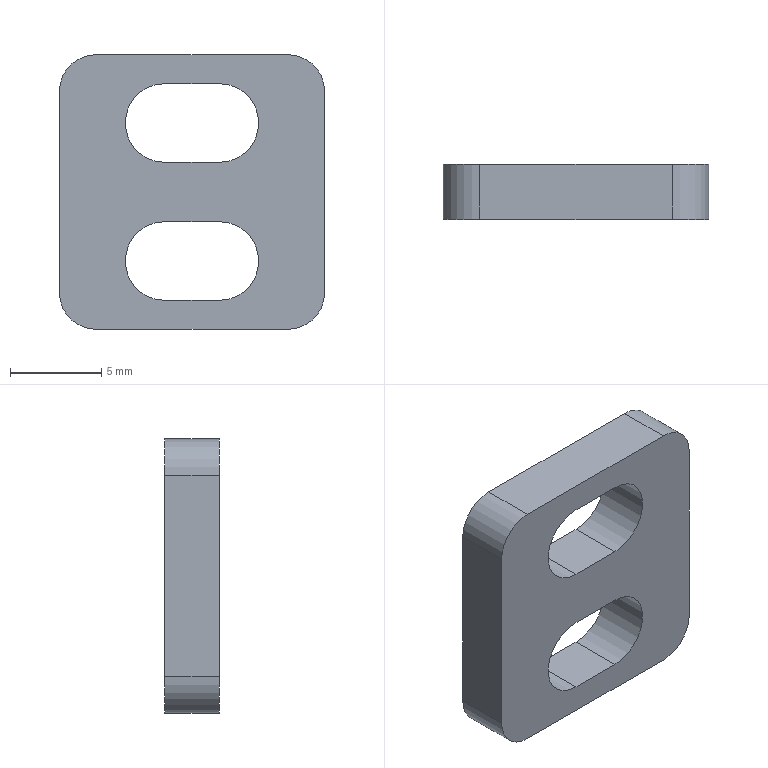Part | SolidWorks | features Extrusion 1, Fillet 1, ICE 1 | 1 solid | 18 faces | box 14.5 x 3 x 15 mm | volume 477.667 mm3 | plane 10 | cylinder 8 | commonest cylinder face diameters 4 x4 4.3 x4
STEP:
#1=CARTESIAN_POINT('',(7.25,0.,5.5));
#2=VERTEX_POINT('',#1);
#3=CARTESIAN_POINT('',(7.25,0.,-5.5));
#4=VERTEX_POINT('',#3);
#5=CARTESIAN_POINT('',(7.25,0.,-7.5));
#6=DIRECTION('',(0.,0.,-1.));
#7=VECTOR('',#6,1000.);
#8=LINE('',#5,#7);
#9=EDGE_CURVE('',#2,#4,#8,.T.);
#10=ORIENTED_EDGE('',*,*,#9,.T.);
#11=CARTESIAN_POINT('',(7.25,3.,-5.5));
#12=VERTEX_POINT('',#11);
#13=CARTESIAN_POINT('',(7.25,3.,-5.5));
#14=DIRECTION('',(0.,1.,0.));
#15=VECTOR('',#14,1000.);
#16=LINE('',#13,#15);
#17=EDGE_CURVE('',#4,#12,#16,.T.);
#18=ORIENTED_EDGE('',*,*,#17,.T.);
#19=CARTESIAN_POINT('',(7.25,3.,5.5));
#20=VERTEX_POINT('',#19);
#21=CARTESIAN_POINT('',(7.25,3.,-7.5));
#22=DIRECTION('',(0.,0.,-1.));
#23=VECTOR('',#22,1000.);
#24=LINE('',#21,#23);
#25=EDGE_CURVE('',#20,#12,#24,.T.);
#26=ORIENTED_EDGE('',*,*,#25,.F.);
#27=CARTESIAN_POINT('',(7.25,3.,5.5));
#28=DIRECTION('',(0.,-1.,0.));
#29=VECTOR('',#28,1000.);
#30=LINE('',#27,#29);
#31=EDGE_CURVE('',#20,#2,#30,.T.);
#32=ORIENTED_EDGE('',*,*,#31,.T.);
#33=EDGE_LOOP('',(#10,#18,#26,#32));
#34=FACE_OUTER_BOUND('',#33,.T.);
#35=CARTESIAN_POINT('',(7.25,3.,-7.5));
#36=DIRECTION('',(-1.,0.,0.));
#37=DIRECTION('',(0.,0.,1.));
#38=AXIS2_PLACEMENT_3D('',#35,#36,#37);
#39=PLANE('',#38);
#40=ADVANCED_FACE('',(#34),#39,.F.);
#41=CARTESIAN_POINT('',(5.25,3.,-7.5));
#42=VERTEX_POINT('',#41);
#43=CARTESIAN_POINT('',(-5.25,3.,-7.5));
#44=VERTEX_POINT('',#43);
#45=CARTESIAN_POINT('',(-7.25,3.,-7.5));
#46=DIRECTION('',(-1.,0.,0.));
#47=VECTOR('',#46,1000.);
#48=LINE('',#45,#47);
#49=EDGE_CURVE('',#42,#44,#48,.T.);
#50=ORIENTED_EDGE('',*,*,#49,.F.);
#51=CARTESIAN_POINT('',(5.25,0.,-7.5));
#52=VERTEX_POINT('',#51);
#53=CARTESIAN_POINT('',(5.25,3.,-7.5));
#54=DIRECTION('',(0.,-1.,0.));
#55=VECTOR('',#54,1000.);
#56=LINE('',#53,#55);
#57=EDGE_CURVE('',#42,#52,#56,.T.);
#58=ORIENTED_EDGE('',*,*,#57,.T.);
#59=CARTESIAN_POINT('',(-5.25,0.,-7.5));
#60=VERTEX_POINT('',#59);
#61=CARTESIAN_POINT('',(-7.25,0.,-7.5));
#62=DIRECTION('',(-1.,0.,0.));
#63=VECTOR('',#62,1000.);
#64=LINE('',#61,#63);
#65=EDGE_CURVE('',#52,#60,#64,.T.);
#66=ORIENTED_EDGE('',*,*,#65,.T.);
#67=CARTESIAN_POINT('',(-5.25,3.,-7.5));
#68=DIRECTION('',(0.,1.,0.));
#69=VECTOR('',#68,1000.);
#70=LINE('',#67,#69);
#71=EDGE_CURVE('',#60,#44,#70,.T.);
#72=ORIENTED_EDGE('',*,*,#71,.T.);
#73=EDGE_LOOP('',(#50,#58,#66,#72));
#74=FACE_OUTER_BOUND('',#73,.T.);
#75=CARTESIAN_POINT('',(-7.25,3.,-7.5));
#76=DIRECTION('',(0.,0.,1.));
#77=DIRECTION('',(1.,0.,0.));
#78=AXIS2_PLACEMENT_3D('',#75,#76,#77);
#79=PLANE('',#78);
#80=ADVANCED_FACE('',(#74),#79,.F.);
#81=CARTESIAN_POINT('',(-7.25,3.,-5.5));
#82=VERTEX_POINT('',#81);
#83=CARTESIAN_POINT('',(-7.25,3.,5.5));
#84=VERTEX_POINT('',#83);
#85=CARTESIAN_POINT('',(-7.25,3.,-7.5));
#86=DIRECTION('',(0.,0.,1.));
#87=VECTOR('',#86,1000.);
#88=LINE('',#85,#87);
#89=EDGE_CURVE('',#82,#84,#88,.T.);
#90=ORIENTED_EDGE('',*,*,#89,.F.);
#91=CARTESIAN_POINT('',(-7.25,0.,-5.5));
#92=VERTEX_POINT('',#91);
#93=CARTESIAN_POINT('',(-7.25,3.,-5.5));
#94=DIRECTION('',(0.,-1.,0.));
#95=VECTOR('',#94,1000.);
#96=LINE('',#93,#95);
#97=EDGE_CURVE('',#82,#92,#96,.T.);
#98=ORIENTED_EDGE('',*,*,#97,.T.);
#99=CARTESIAN_POINT('',(-7.25,0.,5.5));
#100=VERTEX_POINT('',#99);
#101=CARTESIAN_POINT('',(-7.25,0.,-7.5));
#102=DIRECTION('',(0.,0.,1.));
#103=VECTOR('',#102,1000.);
#104=LINE('',#101,#103);
#105=EDGE_CURVE('',#92,#100,#104,.T.);
#106=ORIENTED_EDGE('',*,*,#105,.T.);
#107=CARTESIAN_POINT('',(-7.25,3.,5.5));
#108=DIRECTION('',(0.,1.,0.));
#109=VECTOR('',#108,1000.);
#110=LINE('',#107,#109);
#111=EDGE_CURVE('',#100,#84,#110,.T.);
#112=ORIENTED_EDGE('',*,*,#111,.T.);
#113=EDGE_LOOP('',(#90,#98,#106,#112));
#114=FACE_OUTER_BOUND('',#113,.T.);
#115=CARTESIAN_POINT('',(-7.25,3.,-7.5));
#116=DIRECTION('',(1.,0.,0.));
#117=DIRECTION('',(0.,0.,-1.));
#118=AXIS2_PLACEMENT_3D('',#115,#116,#117);
#119=PLANE('',#118);
#120=ADVANCED_FACE('',(#114),#119,.F.);
#121=CARTESIAN_POINT('',(-5.25,3.,7.5));
#122=VERTEX_POINT('',#121);
#123=CARTESIAN_POINT('',(5.25,3.,7.5));
#124=VERTEX_POINT('',#123);
#125=CARTESIAN_POINT('',(-7.25,3.,7.5));
#126=DIRECTION('',(1.,0.,0.));
#127=VECTOR('',#126,1000.);
#128=LINE('',#125,#127);
#129=EDGE_CURVE('',#122,#124,#128,.T.);
#130=ORIENTED_EDGE('',*,*,#129,.F.);
#131=CARTESIAN_POINT('',(-5.25,0.,7.5));
#132=VERTEX_POINT('',#131);
#133=CARTESIAN_POINT('',(-5.25,3.,7.5));
#134=DIRECTION('',(0.,-1.,0.));
#135=VECTOR('',#134,1000.);
#136=LINE('',#133,#135);
#137=EDGE_CURVE('',#122,#132,#136,.T.);
#138=ORIENTED_EDGE('',*,*,#137,.T.);
#139=CARTESIAN_POINT('',(5.25,0.,7.5));
#140=VERTEX_POINT('',#139);
#141=CARTESIAN_POINT('',(-7.25,0.,7.5));
#142=DIRECTION('',(1.,0.,0.));
#143=VECTOR('',#142,1000.);
#144=LINE('',#141,#143);
#145=EDGE_CURVE('',#132,#140,#144,.T.);
#146=ORIENTED_EDGE('',*,*,#145,.T.);
#147=CARTESIAN_POINT('',(5.25,3.,7.5));
#148=DIRECTION('',(0.,1.,0.));
#149=VECTOR('',#148,1000.);
#150=LINE('',#147,#149);
#151=EDGE_CURVE('',#140,#124,#150,.T.);
#152=ORIENTED_EDGE('',*,*,#151,.T.);
#153=EDGE_LOOP('',(#130,#138,#146,#152));
#154=FACE_OUTER_BOUND('',#153,.T.);
#155=CARTESIAN_POINT('',(-7.25,3.,7.5));
#156=DIRECTION('',(0.,0.,-1.));
#157=DIRECTION('',(-1.,0.,0.));
#158=AXIS2_PLACEMENT_3D('',#155,#156,#157);
#159=PLANE('',#158);
#160=ADVANCED_FACE('',(#154),#159,.F.);
#161=CARTESIAN_POINT('',(1.5,3.,5.922));
#162=VERTEX_POINT('',#161);
#163=CARTESIAN_POINT('',(1.5,3.,1.622));
#164=VERTEX_POINT('',#163);
#165=CARTESIAN_POINT('',(1.5,3.,3.772));
#166=DIRECTION('',(0.,1.,0.));
#167=DIRECTION('',(0.,0.,1.));
#168=AXIS2_PLACEMENT_3D('',#165,#166,#167);
#169=CIRCLE('',#168,2.15);
#170=EDGE_CURVE('',#162,#164,#169,.T.);
#171=ORIENTED_EDGE('',*,*,#170,.F.);
#172=CARTESIAN_POINT('',(-1.5,3.,5.922));
#173=VERTEX_POINT('',#172);
#174=CARTESIAN_POINT('',(0.,3.,5.922));
#175=DIRECTION('',(1.,0.,0.));
#176=VECTOR('',#175,1000.);
#177=LINE('',#174,#176);
#178=EDGE_CURVE('',#173,#162,#177,.T.);
#179=ORIENTED_EDGE('',*,*,#178,.F.);
#180=CARTESIAN_POINT('',(-1.5,3.,1.622));
#181=VERTEX_POINT('',#180);
#182=CARTESIAN_POINT('',(-1.5,3.,3.772));
#183=DIRECTION('',(0.,1.,0.));
#184=DIRECTION('',(0.,0.,1.));
#185=AXIS2_PLACEMENT_3D('',#182,#183,#184);
#186=CIRCLE('',#185,2.15);
#187=EDGE_CURVE('',#181,#173,#186,.T.);
#188=ORIENTED_EDGE('',*,*,#187,.F.);
#189=CARTESIAN_POINT('',(0.,3.,1.622));
#190=DIRECTION('',(-1.,0.,0.));
#191=VECTOR('',#190,1000.);
#192=LINE('',#189,#191);
#193=EDGE_CURVE('',#164,#181,#192,.T.);
#194=ORIENTED_EDGE('',*,*,#193,.F.);
#195=EDGE_LOOP('',(#171,#179,#188,#194));
#196=FACE_BOUND('',#195,.T.);
#197=CARTESIAN_POINT('',(1.5,3.,-1.622));
#198=VERTEX_POINT('',#197);
#199=CARTESIAN_POINT('',(1.5,3.,-5.922));
#200=VERTEX_POINT('',#199);
#201=CARTESIAN_POINT('',(1.5,3.,-3.772));
#202=DIRECTION('',(0.,1.,0.));
#203=DIRECTION('',(0.,0.,1.));
#204=AXIS2_PLACEMENT_3D('',#201,#202,#203);
#205=CIRCLE('',#204,2.15);
#206=EDGE_CURVE('',#198,#200,#205,.T.);
#207=ORIENTED_EDGE('',*,*,#206,.F.);
#208=CARTESIAN_POINT('',(-1.5,3.,-1.622));
#209=VERTEX_POINT('',#208);
#210=CARTESIAN_POINT('',(0.,3.,-1.622));
#211=DIRECTION('',(1.,0.,0.));
#212=VECTOR('',#211,1000.);
#213=LINE('',#210,#212);
#214=EDGE_CURVE('',#209,#198,#213,.T.);
#215=ORIENTED_EDGE('',*,*,#214,.F.);
#216=CARTESIAN_POINT('',(-1.5,3.,-5.922));
#217=VERTEX_POINT('',#216);
#218=CARTESIAN_POINT('',(-1.5,3.,-3.772));
#219=DIRECTION('',(0.,1.,0.));
#220=DIRECTION('',(0.,0.,1.));
#221=AXIS2_PLACEMENT_3D('',#218,#219,#220);
#222=CIRCLE('',#221,2.15);
#223=EDGE_CURVE('',#217,#209,#222,.T.);
#224=ORIENTED_EDGE('',*,*,#223,.F.);
#225=CARTESIAN_POINT('',(0.,3.,-5.922));
#226=DIRECTION('',(-1.,0.,0.));
#227=VECTOR('',#226,1000.);
#228=LINE('',#225,#227);
#229=EDGE_CURVE('',#200,#217,#228,.T.);
#230=ORIENTED_EDGE('',*,*,#229,.F.);
#231=EDGE_LOOP('',(#207,#215,#224,#230));
#232=FACE_BOUND('',#231,.T.);
#233=ORIENTED_EDGE('',*,*,#25,.T.);
#234=CARTESIAN_POINT('',(5.25,3.,-5.5));
#235=DIRECTION('',(0.,1.,0.));
#236=DIRECTION('',(0.,0.,1.));
#237=AXIS2_PLACEMENT_3D('',#234,#235,#236);
#238=CIRCLE('',#237,2.);
#239=EDGE_CURVE('',#12,#42,#238,.T.);
#240=ORIENTED_EDGE('',*,*,#239,.T.);
#241=ORIENTED_EDGE('',*,*,#49,.T.);
#242=CARTESIAN_POINT('',(-5.25,3.,-5.5));
#243=DIRECTION('',(0.,1.,0.));
#244=DIRECTION('',(0.,0.,1.));
#245=AXIS2_PLACEMENT_3D('',#242,#243,#244);
#246=CIRCLE('',#245,2.);
#247=EDGE_CURVE('',#44,#82,#246,.T.);
#248=ORIENTED_EDGE('',*,*,#247,.T.);
#249=ORIENTED_EDGE('',*,*,#89,.T.);
#250=CARTESIAN_POINT('',(-5.25,3.,5.5));
#251=DIRECTION('',(0.,1.,0.));
#252=DIRECTION('',(0.,0.,1.));
#253=AXIS2_PLACEMENT_3D('',#250,#251,#252);
#254=CIRCLE('',#253,2.);
#255=EDGE_CURVE('',#84,#122,#254,.T.);
#256=ORIENTED_EDGE('',*,*,#255,.T.);
#257=ORIENTED_EDGE('',*,*,#129,.T.);
#258=CARTESIAN_POINT('',(5.25,3.,5.5));
#259=DIRECTION('',(0.,1.,0.));
#260=DIRECTION('',(0.,0.,1.));
#261=AXIS2_PLACEMENT_3D('',#258,#259,#260);
#262=CIRCLE('',#261,2.);
#263=EDGE_CURVE('',#124,#20,#262,.T.);
#264=ORIENTED_EDGE('',*,*,#263,.T.);
#265=EDGE_LOOP('',(#233,#240,#241,#248,#249,#256,#257,#264));
#266=FACE_OUTER_BOUND('',#265,.T.);
#267=CARTESIAN_POINT('',(0.,3.,0.));
#268=DIRECTION('',(0.,1.,0.));
#269=DIRECTION('',(0.,0.,1.));
#270=AXIS2_PLACEMENT_3D('',#267,#268,#269);
#271=PLANE('',#270);
#272=ADVANCED_FACE('',(#196,#232,#266),#271,.T.);
#273=CARTESIAN_POINT('',(1.5,0.,5.922));
#274=VERTEX_POINT('',#273);
#275=CARTESIAN_POINT('',(-1.5,0.,5.922));
#276=VERTEX_POINT('',#275);
#277=CARTESIAN_POINT('',(1.5,0.,5.922));
#278=DIRECTION('',(-1.,0.,0.));
#279=VECTOR('',#278,1000.);
#280=LINE('',#277,#279);
#281=EDGE_CURVE('',#274,#276,#280,.T.);
#282=ORIENTED_EDGE('',*,*,#281,.F.);
#283=CARTESIAN_POINT('',(1.5,0.,1.622));
#284=VERTEX_POINT('',#283);
#285=CARTESIAN_POINT('',(1.5,0.,3.772));
#286=DIRECTION('',(0.,-1.,0.));
#287=DIRECTION('',(0.,0.,1.));
#288=AXIS2_PLACEMENT_3D('',#285,#286,#287);
#289=CIRCLE('',#288,2.15);
#290=EDGE_CURVE('',#284,#274,#289,.T.);
#291=ORIENTED_EDGE('',*,*,#290,.F.);
#292=CARTESIAN_POINT('',(-1.5,0.,1.622));
#293=VERTEX_POINT('',#292);
#294=CARTESIAN_POINT('',(1.5,0.,1.622));
#295=DIRECTION('',(1.,0.,0.));
#296=VECTOR('',#295,1000.);
#297=LINE('',#294,#296);
#298=EDGE_CURVE('',#293,#284,#297,.T.);
#299=ORIENTED_EDGE('',*,*,#298,.F.);
#300=CARTESIAN_POINT('',(-1.5,0.,3.772));
#301=DIRECTION('',(0.,-1.,0.));
#302=DIRECTION('',(0.,0.,1.));
#303=AXIS2_PLACEMENT_3D('',#300,#301,#302);
#304=CIRCLE('',#303,2.15);
#305=EDGE_CURVE('',#276,#293,#304,.T.);
#306=ORIENTED_EDGE('',*,*,#305,.F.);
#307=EDGE_LOOP('',(#282,#291,#299,#306));
#308=FACE_BOUND('',#307,.T.);
#309=CARTESIAN_POINT('',(1.5,0.,-1.622));
#310=VERTEX_POINT('',#309);
#311=CARTESIAN_POINT('',(-1.5,0.,-1.622));
#312=VERTEX_POINT('',#311);
#313=CARTESIAN_POINT('',(1.5,0.,-1.622));
#314=DIRECTION('',(-1.,0.,0.));
#315=VECTOR('',#314,1000.);
#316=LINE('',#313,#315);
#317=EDGE_CURVE('',#310,#312,#316,.T.);
#318=ORIENTED_EDGE('',*,*,#317,.F.);
#319=CARTESIAN_POINT('',(1.5,0.,-5.922));
#320=VERTEX_POINT('',#319);
#321=CARTESIAN_POINT('',(1.5,0.,-3.772));
#322=DIRECTION('',(0.,-1.,0.));
#323=DIRECTION('',(0.,0.,-1.));
#324=AXIS2_PLACEMENT_3D('',#321,#322,#323);
#325=CIRCLE('',#324,2.15);
#326=EDGE_CURVE('',#320,#310,#325,.T.);
#327=ORIENTED_EDGE('',*,*,#326,.F.);
#328=CARTESIAN_POINT('',(-1.5,0.,-5.922));
#329=VERTEX_POINT('',#328);
#330=CARTESIAN_POINT('',(1.5,0.,-5.922));
#331=DIRECTION('',(1.,0.,0.));
#332=VECTOR('',#331,1000.);
#333=LINE('',#330,#332);
#334=EDGE_CURVE('',#329,#320,#333,.T.);
#335=ORIENTED_EDGE('',*,*,#334,.F.);
#336=CARTESIAN_POINT('',(-1.5,0.,-3.772));
#337=DIRECTION('',(0.,-1.,0.));
#338=DIRECTION('',(0.,0.,-1.));
#339=AXIS2_PLACEMENT_3D('',#336,#337,#338);
#340=CIRCLE('',#339,2.15);
#341=EDGE_CURVE('',#312,#329,#340,.T.);
#342=ORIENTED_EDGE('',*,*,#341,.F.);
#343=EDGE_LOOP('',(#318,#327,#335,#342));
#344=FACE_BOUND('',#343,.T.);
#345=ORIENTED_EDGE('',*,*,#65,.F.);
#346=CARTESIAN_POINT('',(5.25,0.,-5.5));
#347=DIRECTION('',(0.,-1.,0.));
#348=DIRECTION('',(0.,0.,1.));
#349=AXIS2_PLACEMENT_3D('',#346,#347,#348);
#350=CIRCLE('',#349,2.);
#351=EDGE_CURVE('',#52,#4,#350,.T.);
#352=ORIENTED_EDGE('',*,*,#351,.T.);
#353=ORIENTED_EDGE('',*,*,#9,.F.);
#354=CARTESIAN_POINT('',(5.25,0.,5.5));
#355=DIRECTION('',(0.,-1.,0.));
#356=DIRECTION('',(0.,0.,1.));
#357=AXIS2_PLACEMENT_3D('',#354,#355,#356);
#358=CIRCLE('',#357,2.);
#359=EDGE_CURVE('',#2,#140,#358,.T.);
#360=ORIENTED_EDGE('',*,*,#359,.T.);
#361=ORIENTED_EDGE('',*,*,#145,.F.);
#362=CARTESIAN_POINT('',(-5.25,0.,5.5));
#363=DIRECTION('',(0.,-1.,0.));
#364=DIRECTION('',(0.,0.,1.));
#365=AXIS2_PLACEMENT_3D('',#362,#363,#364);
#366=CIRCLE('',#365,2.);
#367=EDGE_CURVE('',#132,#100,#366,.T.);
#368=ORIENTED_EDGE('',*,*,#367,.T.);
#369=ORIENTED_EDGE('',*,*,#105,.F.);
#370=CARTESIAN_POINT('',(-5.25,0.,-5.5));
#371=DIRECTION('',(0.,-1.,0.));
#372=DIRECTION('',(0.,0.,1.));
#373=AXIS2_PLACEMENT_3D('',#370,#371,#372);
#374=CIRCLE('',#373,2.);
#375=EDGE_CURVE('',#92,#60,#374,.T.);
#376=ORIENTED_EDGE('',*,*,#375,.T.);
#377=EDGE_LOOP('',(#345,#352,#353,#360,#361,#368,#369,#376));
#378=FACE_OUTER_BOUND('',#377,.T.);
#379=CARTESIAN_POINT('',(0.,0.,0.));
#380=DIRECTION('',(0.,1.,0.));
#381=DIRECTION('',(0.,0.,1.));
#382=AXIS2_PLACEMENT_3D('',#379,#380,#381);
#383=PLANE('',#382);
#384=ADVANCED_FACE('',(#308,#344,#378),#383,.F.);
#385=ORIENTED_EDGE('',*,*,#206,.T.);
#386=CARTESIAN_POINT('',(1.5,10.,-5.922));
#387=DIRECTION('',(0.,-1.,0.));
#388=VECTOR('',#387,1000.);
#389=LINE('',#386,#388);
#390=EDGE_CURVE('',#200,#320,#389,.T.);
#391=ORIENTED_EDGE('',*,*,#390,.T.);
#392=ORIENTED_EDGE('',*,*,#326,.T.);
#393=CARTESIAN_POINT('',(1.5,10.,-1.622));
#394=DIRECTION('',(0.,-1.,0.));
#395=VECTOR('',#394,1000.);
#396=LINE('',#393,#395);
#397=EDGE_CURVE('',#198,#310,#396,.T.);
#398=ORIENTED_EDGE('',*,*,#397,.F.);
#399=EDGE_LOOP('',(#385,#391,#392,#398));
#400=FACE_OUTER_BOUND('',#399,.T.);
#401=CARTESIAN_POINT('',(1.5,10.,-3.772));
#402=DIRECTION('',(0.,-1.,0.));
#403=DIRECTION('',(0.,0.,-1.));
#404=AXIS2_PLACEMENT_3D('',#401,#402,#403);
#405=CYLINDRICAL_SURFACE('',#404,2.15);
#406=ADVANCED_FACE('',(#400),#405,.F.);
#407=ORIENTED_EDGE('',*,*,#229,.T.);
#408=CARTESIAN_POINT('',(-1.5,10.,-5.922));
#409=DIRECTION('',(0.,-1.,0.));
#410=VECTOR('',#409,1000.);
#411=LINE('',#408,#410);
#412=EDGE_CURVE('',#217,#329,#411,.T.);
#413=ORIENTED_EDGE('',*,*,#412,.T.);
#414=ORIENTED_EDGE('',*,*,#334,.T.);
#415=ORIENTED_EDGE('',*,*,#390,.F.);
#416=EDGE_LOOP('',(#407,#413,#414,#415));
#417=FACE_OUTER_BOUND('',#416,.T.);
#418=CARTESIAN_POINT('',(1.5,10.,-5.922));
#419=DIRECTION('',(0.,0.,-1.));
#420=DIRECTION('',(-1.,0.,0.));
#421=AXIS2_PLACEMENT_3D('',#418,#419,#420);
#422=PLANE('',#421);
#423=ADVANCED_FACE('',(#417),#422,.F.);
#424=ORIENTED_EDGE('',*,*,#223,.T.);
#425=CARTESIAN_POINT('',(-1.5,10.,-1.622));
#426=DIRECTION('',(0.,-1.,0.));
#427=VECTOR('',#426,1000.);
#428=LINE('',#425,#427);
#429=EDGE_CURVE('',#209,#312,#428,.T.);
#430=ORIENTED_EDGE('',*,*,#429,.T.);
#431=ORIENTED_EDGE('',*,*,#341,.T.);
#432=ORIENTED_EDGE('',*,*,#412,.F.);
#433=EDGE_LOOP('',(#424,#430,#431,#432));
#434=FACE_OUTER_BOUND('',#433,.T.);
#435=CARTESIAN_POINT('',(-1.5,10.,-3.772));
#436=DIRECTION('',(0.,-1.,0.));
#437=DIRECTION('',(0.,0.,-1.));
#438=AXIS2_PLACEMENT_3D('',#435,#436,#437);
#439=CYLINDRICAL_SURFACE('',#438,2.15);
#440=ADVANCED_FACE('',(#434),#439,.F.);
#441=ORIENTED_EDGE('',*,*,#214,.T.);
#442=ORIENTED_EDGE('',*,*,#397,.T.);
#443=ORIENTED_EDGE('',*,*,#317,.T.);
#444=ORIENTED_EDGE('',*,*,#429,.F.);
#445=EDGE_LOOP('',(#441,#442,#443,#444));
#446=FACE_OUTER_BOUND('',#445,.T.);
#447=CARTESIAN_POINT('',(1.5,10.,-1.622));
#448=DIRECTION('',(0.,0.,1.));
#449=DIRECTION('',(1.,0.,0.));
#450=AXIS2_PLACEMENT_3D('',#447,#448,#449);
#451=PLANE('',#450);
#452=ADVANCED_FACE('',(#446),#451,.F.);
#453=ORIENTED_EDGE('',*,*,#170,.T.);
#454=CARTESIAN_POINT('',(1.5,10.,1.622));
#455=DIRECTION('',(0.,-1.,0.));
#456=VECTOR('',#455,1000.);
#457=LINE('',#454,#456);
#458=EDGE_CURVE('',#164,#284,#457,.T.);
#459=ORIENTED_EDGE('',*,*,#458,.T.);
#460=ORIENTED_EDGE('',*,*,#290,.T.);
#461=CARTESIAN_POINT('',(1.5,10.,5.922));
#462=DIRECTION('',(0.,-1.,0.));
#463=VECTOR('',#462,1000.);
#464=LINE('',#461,#463);
#465=EDGE_CURVE('',#162,#274,#464,.T.);
#466=ORIENTED_EDGE('',*,*,#465,.F.);
#467=EDGE_LOOP('',(#453,#459,#460,#466));
#468=FACE_OUTER_BOUND('',#467,.T.);
#469=CARTESIAN_POINT('',(1.5,10.,3.772));
#470=DIRECTION('',(0.,-1.,0.));
#471=DIRECTION('',(0.,0.,-1.));
#472=AXIS2_PLACEMENT_3D('',#469,#470,#471);
#473=CYLINDRICAL_SURFACE('',#472,2.15);
#474=ADVANCED_FACE('',(#468),#473,.F.);
#475=ORIENTED_EDGE('',*,*,#193,.T.);
#476=CARTESIAN_POINT('',(-1.5,10.,1.622));
#477=DIRECTION('',(0.,-1.,0.));
#478=VECTOR('',#477,1000.);
#479=LINE('',#476,#478);
#480=EDGE_CURVE('',#181,#293,#479,.T.);
#481=ORIENTED_EDGE('',*,*,#480,.T.);
#482=ORIENTED_EDGE('',*,*,#298,.T.);
#483=ORIENTED_EDGE('',*,*,#458,.F.);
#484=EDGE_LOOP('',(#475,#481,#482,#483));
#485=FACE_OUTER_BOUND('',#484,.T.);
#486=CARTESIAN_POINT('',(1.5,10.,1.622));
#487=DIRECTION('',(0.,0.,-1.));
#488=DIRECTION('',(-1.,0.,0.));
#489=AXIS2_PLACEMENT_3D('',#486,#487,#488);
#490=PLANE('',#489);
#491=ADVANCED_FACE('',(#485),#490,.F.);
#492=ORIENTED_EDGE('',*,*,#187,.T.);
#493=CARTESIAN_POINT('',(-1.5,10.,5.922));
#494=DIRECTION('',(0.,-1.,0.));
#495=VECTOR('',#494,1000.);
#496=LINE('',#493,#495);
#497=EDGE_CURVE('',#173,#276,#496,.T.);
#498=ORIENTED_EDGE('',*,*,#497,.T.);
#499=ORIENTED_EDGE('',*,*,#305,.T.);
#500=ORIENTED_EDGE('',*,*,#480,.F.);
#501=EDGE_LOOP('',(#492,#498,#499,#500));
#502=FACE_OUTER_BOUND('',#501,.T.);
#503=CARTESIAN_POINT('',(-1.5,10.,3.772));
#504=DIRECTION('',(0.,-1.,0.));
#505=DIRECTION('',(0.,0.,-1.));
#506=AXIS2_PLACEMENT_3D('',#503,#504,#505);
#507=CYLINDRICAL_SURFACE('',#506,2.15);
#508=ADVANCED_FACE('',(#502),#507,.F.);
#509=ORIENTED_EDGE('',*,*,#178,.T.);
#510=ORIENTED_EDGE('',*,*,#465,.T.);
#511=ORIENTED_EDGE('',*,*,#281,.T.);
#512=ORIENTED_EDGE('',*,*,#497,.F.);
#513=EDGE_LOOP('',(#509,#510,#511,#512));
#514=FACE_OUTER_BOUND('',#513,.T.);
#515=CARTESIAN_POINT('',(1.5,10.,5.922));
#516=DIRECTION('',(0.,0.,1.));
#517=DIRECTION('',(1.,0.,0.));
#518=AXIS2_PLACEMENT_3D('',#515,#516,#517);
#519=PLANE('',#518);
#520=ADVANCED_FACE('',(#514),#519,.F.);
#521=ORIENTED_EDGE('',*,*,#239,.F.);
#522=ORIENTED_EDGE('',*,*,#17,.F.);
#523=ORIENTED_EDGE('',*,*,#351,.F.);
#524=ORIENTED_EDGE('',*,*,#57,.F.);
#525=EDGE_LOOP('',(#521,#522,#523,#524));
#526=FACE_OUTER_BOUND('',#525,.T.);
#527=CARTESIAN_POINT('',(5.25,3.,-5.5));
#528=DIRECTION('',(0.,-1.,0.));
#529=DIRECTION('',(0.,0.,-1.));
#530=AXIS2_PLACEMENT_3D('',#527,#528,#529);
#531=CYLINDRICAL_SURFACE('',#530,2.);
#532=ADVANCED_FACE('',(#526),#531,.T.);
#533=ORIENTED_EDGE('',*,*,#247,.F.);
#534=ORIENTED_EDGE('',*,*,#71,.F.);
#535=ORIENTED_EDGE('',*,*,#375,.F.);
#536=ORIENTED_EDGE('',*,*,#97,.F.);
#537=EDGE_LOOP('',(#533,#534,#535,#536));
#538=FACE_OUTER_BOUND('',#537,.T.);
#539=CARTESIAN_POINT('',(-5.25,3.,-5.5));
#540=DIRECTION('',(0.,-1.,0.));
#541=DIRECTION('',(0.,0.,-1.));
#542=AXIS2_PLACEMENT_3D('',#539,#540,#541);
#543=CYLINDRICAL_SURFACE('',#542,2.);
#544=ADVANCED_FACE('',(#538),#543,.T.);
#545=ORIENTED_EDGE('',*,*,#255,.F.);
#546=ORIENTED_EDGE('',*,*,#111,.F.);
#547=ORIENTED_EDGE('',*,*,#367,.F.);
#548=ORIENTED_EDGE('',*,*,#137,.F.);
#549=EDGE_LOOP('',(#545,#546,#547,#548));
#550=FACE_OUTER_BOUND('',#549,.T.);
#551=CARTESIAN_POINT('',(-5.25,3.,5.5));
#552=DIRECTION('',(0.,-1.,0.));
#553=DIRECTION('',(0.,0.,-1.));
#554=AXIS2_PLACEMENT_3D('',#551,#552,#553);
#555=CYLINDRICAL_SURFACE('',#554,2.);
#556=ADVANCED_FACE('',(#550),#555,.T.);
#557=ORIENTED_EDGE('',*,*,#263,.F.);
#558=ORIENTED_EDGE('',*,*,#151,.F.);
#559=ORIENTED_EDGE('',*,*,#359,.F.);
#560=ORIENTED_EDGE('',*,*,#31,.F.);
#561=EDGE_LOOP('',(#557,#558,#559,#560));
#562=FACE_OUTER_BOUND('',#561,.T.);
#563=CARTESIAN_POINT('',(5.25,3.,5.5));
#564=DIRECTION('',(0.,-1.,0.));
#565=DIRECTION('',(0.,0.,-1.));
#566=AXIS2_PLACEMENT_3D('',#563,#564,#565);
#567=CYLINDRICAL_SURFACE('',#566,2.);
#568=ADVANCED_FACE('',(#562),#567,.T.);
#569=CLOSED_SHELL('',(#40,#80,#120,#160,#272,#384,#406,#423,#440,#452,#474,#491,#508,#520,#532,#544,#556,#568));
#570=MANIFOLD_SOLID_BREP('',#569);
#571=CARTESIAN_POINT('',(0.,0.,0.));
#572=DIRECTION('',(0.,0.,1.));
#573=DIRECTION('',(1.,0.,0.));
#574=AXIS2_PLACEMENT_3D('',#571,#572,#573);
#575=(LENGTH_UNIT()NAMED_UNIT(*)SI_UNIT(.MILLI.,.METRE.));
#576=UNCERTAINTY_MEASURE_WITH_UNIT(LENGTH_MEASURE(0.00001),#575,'','');
#577=(NAMED_UNIT(*)PLANE_ANGLE_UNIT()SI_UNIT($,.RADIAN.));
#578=(NAMED_UNIT(*)SI_UNIT($,.STERADIAN.)SOLID_ANGLE_UNIT());
#579=(GEOMETRIC_REPRESENTATION_CONTEXT(3)GLOBAL_UNCERTAINTY_ASSIGNED_CONTEXT((#576))GLOBAL_UNIT_ASSIGNED_CONTEXT((#575,#577,#578))REPRESENTATION_CONTEXT('',''));
#580=ADVANCED_BREP_SHAPE_REPRESENTATION('',(#570,#574),#579);